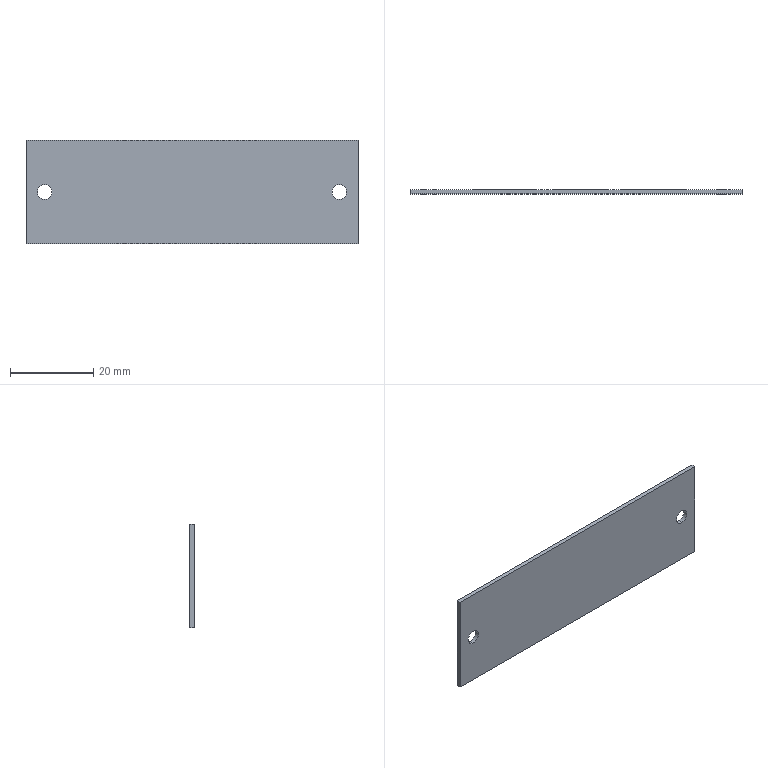Part | SolidWorks | features Extrusion 1, ICE 1 | 1 solid | 362 faces | box 80 x 1 x 25 mm | volume 1928 mm3 | plane 263 | spline 95 | cylinder 4 | commonest cylinder face diameters 3.5 x4